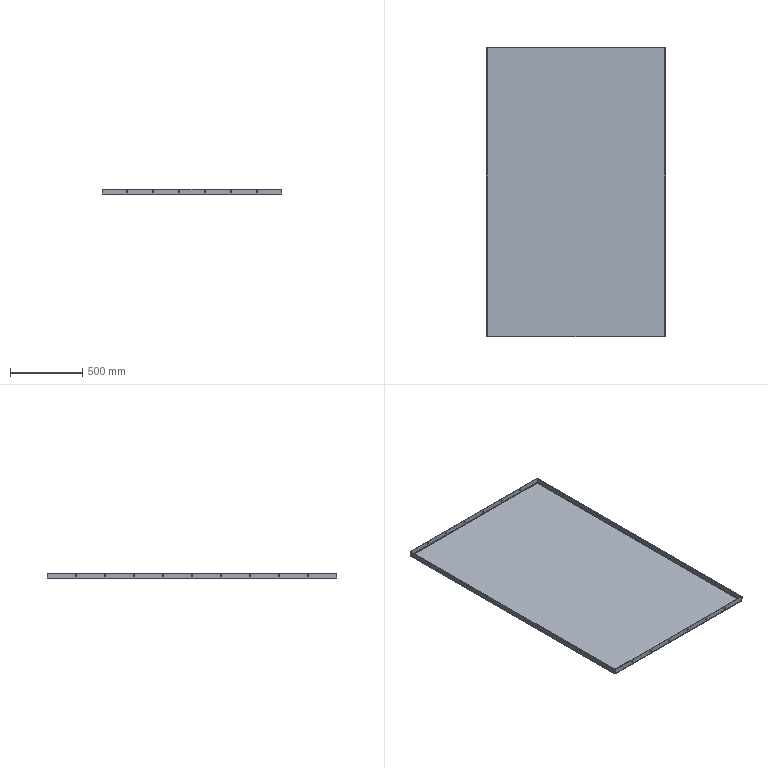Part | SolidWorks | features ICE 2, CornerFeat 1, EdgeFlange 1, FlatPattern 1, SMBaseFlange 1, SheetMetal 1 | 1 solid | 98 faces | box 1240 x 2000 x 40 mm | volume 8113191 mm3 | cylinder 68 | plane 22 | spline 8 | commonest cylinder face diameters 10 x60 6 x4 12 x4